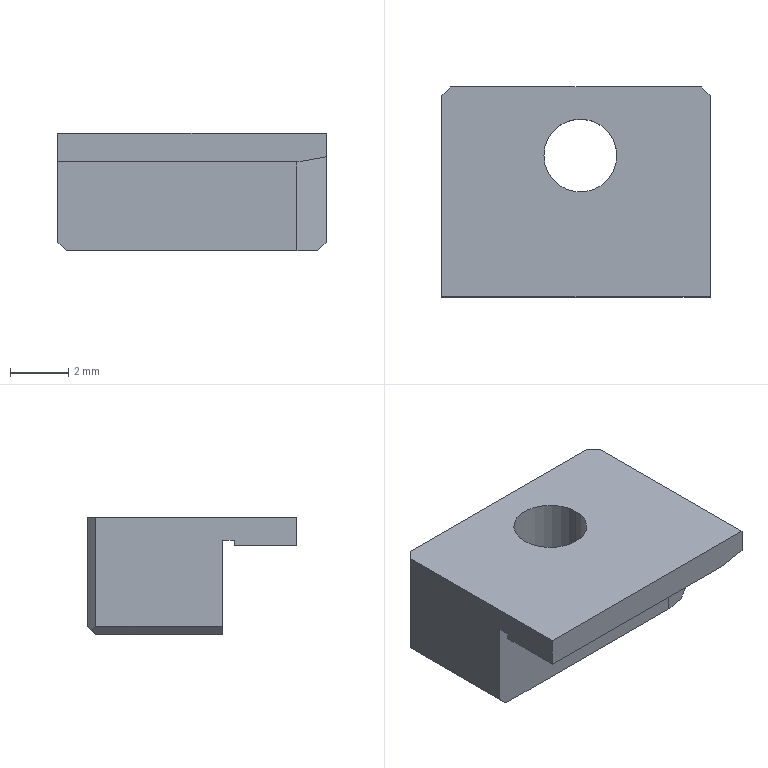Part | NX | 1 solid | 22 faces | box 9.2 x 7.2 x 4.04 mm | volume 173.358 mm3 | plane 18 | cylinder 2 | cone 2 | commonest cylinder face diameters 2.5 x2
STEP:
#1=CARTESIAN_POINT('',(-39.91,-38.279,0.4031));
#2=VERTEX_POINT('',#1);
#3=CARTESIAN_POINT('',(-39.91,-38.279,3.453));
#4=VERTEX_POINT('',#3);
#5=CARTESIAN_POINT('',(-39.91,-38.279,1.928));
#6=DIRECTION('',(0.,0.,1.));
#7=VECTOR('',#6,1000.);
#8=LINE('',#5,#7);
#9=EDGE_CURVE('',#2,#4,#8,.T.);
#10=ORIENTED_EDGE('',*,*,#9,.T.);
#11=CARTESIAN_POINT('',(-38.91,-38.279,3.629));
#12=VERTEX_POINT('',#11);
#13=CARTESIAN_POINT('',(-41.256,-38.279,3.216));
#14=DIRECTION('',(-0.9848,0.,-0.1736));
#15=VECTOR('',#14,1000.);
#16=LINE('',#13,#15);
#17=EDGE_CURVE('',#12,#4,#16,.T.);
#18=ORIENTED_EDGE('',*,*,#17,.F.);
#19=CARTESIAN_POINT('',(-38.91,-38.279,3.653));
#20=VERTEX_POINT('',#19);
#21=CARTESIAN_POINT('',(-38.91,-38.279,3.403));
#22=DIRECTION('',(0.,0.,1.));
#23=VECTOR('',#22,1000.);
#24=LINE('',#21,#23);
#25=EDGE_CURVE('',#12,#20,#24,.T.);
#26=ORIENTED_EDGE('',*,*,#25,.T.);
#27=CARTESIAN_POINT('',(-48.11,-38.279,3.653));
#28=VERTEX_POINT('',#27);
#29=CARTESIAN_POINT('',(-37.99,-38.279,3.653));
#30=DIRECTION('',(-1.,0.,0.));
#31=VECTOR('',#30,1000.);
#32=LINE('',#29,#31);
#33=EDGE_CURVE('',#20,#28,#32,.T.);
#34=ORIENTED_EDGE('',*,*,#33,.T.);
#35=CARTESIAN_POINT('',(-48.11,-38.279,0.7031));
#36=VERTEX_POINT('',#35);
#37=CARTESIAN_POINT('',(-48.11,-38.279,3.403));
#38=DIRECTION('',(0.,0.,1.));
#39=VECTOR('',#38,1000.);
#40=LINE('',#37,#39);
#41=EDGE_CURVE('',#36,#28,#40,.T.);
#42=ORIENTED_EDGE('',*,*,#41,.F.);
#43=CARTESIAN_POINT('',(-47.81,-38.279,0.4031));
#44=VERTEX_POINT('',#43);
#45=CARTESIAN_POINT('',(-50.81,-38.279,3.403));
#46=DIRECTION('',(-0.7071,0.,0.7071));
#47=VECTOR('',#46,1000.);
#48=LINE('',#45,#47);
#49=EDGE_CURVE('',#44,#36,#48,.T.);
#50=ORIENTED_EDGE('',*,*,#49,.F.);
#51=CARTESIAN_POINT('',(-41.256,-38.279,0.4031));
#52=DIRECTION('',(-1.,0.,0.));
#53=VECTOR('',#52,1000.);
#54=LINE('',#51,#53);
#55=EDGE_CURVE('',#2,#44,#54,.T.);
#56=ORIENTED_EDGE('',*,*,#55,.F.);
#57=EDGE_LOOP('',(#10,#18,#26,#34,#42,#50,#56));
#58=FACE_BOUND('',#57,.T.);
#59=CARTESIAN_POINT('',(-48.11,-38.279,3.403));
#60=DIRECTION('',(0.,-1.,0.));
#61=DIRECTION('',(-1.,0.,0.));
#62=AXIS2_PLACEMENT_3D('',#59,#60,#61);
#63=PLANE('',#62);
#64=ADVANCED_FACE('',(#58),#63,.T.);
#65=CARTESIAN_POINT('',(-48.11,-33.929,4.443));
#66=VERTEX_POINT('',#65);
#67=CARTESIAN_POINT('',(-48.11,-40.829,4.443));
#68=VERTEX_POINT('',#67);
#69=CARTESIAN_POINT('',(-48.11,-36.022,4.443));
#70=DIRECTION('',(0.,-1.,0.));
#71=VECTOR('',#70,1000.);
#72=LINE('',#69,#71);
#73=EDGE_CURVE('',#66,#68,#72,.T.);
#74=ORIENTED_EDGE('',*,*,#73,.F.);
#75=CARTESIAN_POINT('',(-48.11,-33.929,0.7031));
#76=VERTEX_POINT('',#75);
#77=CARTESIAN_POINT('',(-48.11,-33.929,3.403));
#78=DIRECTION('',(0.,0.,-1.));
#79=VECTOR('',#78,1000.);
#80=LINE('',#77,#79);
#81=EDGE_CURVE('',#66,#76,#80,.T.);
#82=ORIENTED_EDGE('',*,*,#81,.T.);
#83=CARTESIAN_POINT('',(-48.11,-36.022,0.7031));
#84=DIRECTION('',(0.,1.,0.));
#85=VECTOR('',#84,1000.);
#86=LINE('',#83,#85);
#87=EDGE_CURVE('',#36,#76,#86,.T.);
#88=ORIENTED_EDGE('',*,*,#87,.F.);
#89=ORIENTED_EDGE('',*,*,#41,.T.);
#90=CARTESIAN_POINT('',(-48.11,-38.679,3.653));
#91=VERTEX_POINT('',#90);
#92=CARTESIAN_POINT('',(-48.11,-36.022,3.653));
#93=DIRECTION('',(0.,1.,0.));
#94=VECTOR('',#93,1000.);
#95=LINE('',#92,#94);
#96=EDGE_CURVE('',#91,#28,#95,.T.);
#97=ORIENTED_EDGE('',*,*,#96,.F.);
#98=CARTESIAN_POINT('',(-48.11,-38.679,3.453));
#99=VERTEX_POINT('',#98);
#100=CARTESIAN_POINT('',(-48.11,-38.679,3.403));
#101=DIRECTION('',(0.,0.,1.));
#102=VECTOR('',#101,1000.);
#103=LINE('',#100,#102);
#104=EDGE_CURVE('',#99,#91,#103,.T.);
#105=ORIENTED_EDGE('',*,*,#104,.F.);
#106=CARTESIAN_POINT('',(-48.11,-40.829,3.453));
#107=VERTEX_POINT('',#106);
#108=CARTESIAN_POINT('',(-48.11,-36.022,3.453));
#109=DIRECTION('',(0.,-1.,0.));
#110=VECTOR('',#109,1000.);
#111=LINE('',#108,#110);
#112=EDGE_CURVE('',#99,#107,#111,.T.);
#113=ORIENTED_EDGE('',*,*,#112,.T.);
#114=CARTESIAN_POINT('',(-48.11,-40.829,3.403));
#115=DIRECTION('',(0.,0.,1.));
#116=VECTOR('',#115,1000.);
#117=LINE('',#114,#116);
#118=EDGE_CURVE('',#107,#68,#117,.T.);
#119=ORIENTED_EDGE('',*,*,#118,.T.);
#120=EDGE_LOOP('',(#74,#82,#88,#89,#97,#105,#113,#119));
#121=FACE_BOUND('',#120,.T.);
#122=CARTESIAN_POINT('',(-48.11,-31.629,3.403));
#123=DIRECTION('',(-1.,0.,0.));
#124=DIRECTION('',(0.,1.,0.));
#125=AXIS2_PLACEMENT_3D('',#122,#123,#124);
#126=PLANE('',#125);
#127=ADVANCED_FACE('',(#121),#126,.T.);
#128=CARTESIAN_POINT('',(-39.21,-33.629,4.443));
#129=VERTEX_POINT('',#128);
#130=CARTESIAN_POINT('',(-39.21,-33.629,0.7031));
#131=VERTEX_POINT('',#130);
#132=CARTESIAN_POINT('',(-39.21,-33.629,3.403));
#133=DIRECTION('',(0.,0.,-1.));
#134=VECTOR('',#133,1000.);
#135=LINE('',#132,#134);
#136=EDGE_CURVE('',#129,#131,#135,.T.);
#137=ORIENTED_EDGE('',*,*,#136,.T.);
#138=CARTESIAN_POINT('',(-47.81,-33.629,0.7031));
#139=VERTEX_POINT('',#138);
#140=CARTESIAN_POINT('',(-41.256,-33.629,0.7031));
#141=DIRECTION('',(-1.,0.,0.));
#142=VECTOR('',#141,1000.);
#143=LINE('',#140,#142);
#144=EDGE_CURVE('',#131,#139,#143,.T.);
#145=ORIENTED_EDGE('',*,*,#144,.T.);
#146=CARTESIAN_POINT('',(-47.81,-33.629,4.443));
#147=VERTEX_POINT('',#146);
#148=CARTESIAN_POINT('',(-47.81,-33.629,3.403));
#149=DIRECTION('',(0.,0.,-1.));
#150=VECTOR('',#149,1000.);
#151=LINE('',#148,#150);
#152=EDGE_CURVE('',#147,#139,#151,.T.);
#153=ORIENTED_EDGE('',*,*,#152,.F.);
#154=CARTESIAN_POINT('',(-41.256,-33.629,4.443));
#155=DIRECTION('',(-1.,0.,0.));
#156=VECTOR('',#155,1000.);
#157=LINE('',#154,#156);
#158=EDGE_CURVE('',#129,#147,#157,.T.);
#159=ORIENTED_EDGE('',*,*,#158,.F.);
#160=EDGE_LOOP('',(#137,#145,#153,#159));
#161=FACE_BOUND('',#160,.T.);
#162=CARTESIAN_POINT('',(-38.61,-33.629,3.403));
#163=DIRECTION('',(0.,1.,0.));
#164=DIRECTION('',(1.,0.,0.));
#165=AXIS2_PLACEMENT_3D('',#162,#163,#164);
#166=PLANE('',#165);
#167=ADVANCED_FACE('',(#161),#166,.T.);
#168=CARTESIAN_POINT('',(-38.91,-38.679,3.629));
#169=VERTEX_POINT('',#168);
#170=CARTESIAN_POINT('',(-38.91,-40.829,3.629));
#171=VERTEX_POINT('',#170);
#172=CARTESIAN_POINT('',(-38.91,-39.554,3.629));
#173=DIRECTION('',(0.,-1.,0.));
#174=VECTOR('',#173,1000.);
#175=LINE('',#172,#174);
#176=EDGE_CURVE('',#169,#171,#175,.T.);
#177=ORIENTED_EDGE('',*,*,#176,.F.);
#178=CARTESIAN_POINT('',(-38.91,-38.679,3.653));
#179=VERTEX_POINT('',#178);
#180=CARTESIAN_POINT('',(-38.91,-38.679,3.403));
#181=DIRECTION('',(0.,0.,-1.));
#182=VECTOR('',#181,1000.);
#183=LINE('',#180,#182);
#184=EDGE_CURVE('',#179,#169,#183,.T.);
#185=ORIENTED_EDGE('',*,*,#184,.F.);
#186=CARTESIAN_POINT('',(-38.91,-36.022,3.653));
#187=DIRECTION('',(0.,-1.,0.));
#188=VECTOR('',#187,1000.);
#189=LINE('',#186,#188);
#190=EDGE_CURVE('',#20,#179,#189,.T.);
#191=ORIENTED_EDGE('',*,*,#190,.F.);
#192=ORIENTED_EDGE('',*,*,#25,.F.);
#193=CARTESIAN_POINT('',(-38.91,-38.103,3.629));
#194=VERTEX_POINT('',#193);
#195=CARTESIAN_POINT('',(-38.91,-39.554,3.629));
#196=DIRECTION('',(0.,-1.,0.));
#197=VECTOR('',#196,1000.);
#198=LINE('',#195,#197);
#199=EDGE_CURVE('',#194,#12,#198,.T.);
#200=ORIENTED_EDGE('',*,*,#199,.F.);
#201=CARTESIAN_POINT('',(-38.91,-38.103,0.7031));
#202=VERTEX_POINT('',#201);
#203=CARTESIAN_POINT('',(-38.91,-38.103,1.928));
#204=DIRECTION('',(0.,0.,1.));
#205=VECTOR('',#204,1000.);
#206=LINE('',#203,#205);
#207=EDGE_CURVE('',#202,#194,#206,.T.);
#208=ORIENTED_EDGE('',*,*,#207,.F.);
#209=CARTESIAN_POINT('',(-38.91,-33.929,0.7031));
#210=VERTEX_POINT('',#209);
#211=CARTESIAN_POINT('',(-38.91,-36.104,0.7031));
#212=DIRECTION('',(0.,-1.,0.));
#213=VECTOR('',#212,1000.);
#214=LINE('',#211,#213);
#215=EDGE_CURVE('',#210,#202,#214,.T.);
#216=ORIENTED_EDGE('',*,*,#215,.F.);
#217=CARTESIAN_POINT('',(-38.91,-33.929,4.443));
#218=VERTEX_POINT('',#217);
#219=CARTESIAN_POINT('',(-38.91,-33.929,3.403));
#220=DIRECTION('',(0.,0.,-1.));
#221=VECTOR('',#220,1000.);
#222=LINE('',#219,#221);
#223=EDGE_CURVE('',#218,#210,#222,.T.);
#224=ORIENTED_EDGE('',*,*,#223,.F.);
#225=CARTESIAN_POINT('',(-38.91,-40.829,4.443));
#226=VERTEX_POINT('',#225);
#227=CARTESIAN_POINT('',(-38.91,-36.022,4.443));
#228=DIRECTION('',(0.,1.,0.));
#229=VECTOR('',#228,1000.);
#230=LINE('',#227,#229);
#231=EDGE_CURVE('',#226,#218,#230,.T.);
#232=ORIENTED_EDGE('',*,*,#231,.F.);
#233=CARTESIAN_POINT('',(-38.91,-40.829,3.403));
#234=DIRECTION('',(0.,0.,1.));
#235=VECTOR('',#234,1000.);
#236=LINE('',#233,#235);
#237=EDGE_CURVE('',#171,#226,#236,.T.);
#238=ORIENTED_EDGE('',*,*,#237,.F.);
#239=EDGE_LOOP('',(#177,#185,#191,#192,#200,#208,#216,#224,#232,#238));
#240=FACE_BOUND('',#239,.T.);
#241=CARTESIAN_POINT('',(-38.91,-38.329,3.403));
#242=DIRECTION('',(1.,0.,0.));
#243=DIRECTION('',(0.,0.,1.));
#244=AXIS2_PLACEMENT_3D('',#241,#242,#243);
#245=PLANE('',#244);
#246=ADVANCED_FACE('',(#240),#245,.T.);
#247=CARTESIAN_POINT('',(-41.256,-27.074,4.443));
#248=DIRECTION('',(-0.7071,-0.7071,0.));
#249=VECTOR('',#248,1000.);
#250=LINE('',#247,#249);
#251=EDGE_CURVE('',#147,#66,#250,.T.);
#252=ORIENTED_EDGE('',*,*,#251,.F.);
#253=ORIENTED_EDGE('',*,*,#152,.T.);
#254=CARTESIAN_POINT('',(-47.96,-33.779,0.5531));
#255=VERTEX_POINT('',#254);
#256=CARTESIAN_POINT('',(-41.256,-27.074,7.258));
#257=DIRECTION('',(-0.5774,-0.5774,-0.5774));
#258=VECTOR('',#257,1000.);
#259=LINE('',#256,#258);
#260=EDGE_CURVE('',#139,#255,#259,.T.);
#261=ORIENTED_EDGE('',*,*,#260,.T.);
#262=CARTESIAN_POINT('',(-50.81,-36.629,3.403));
#263=DIRECTION('',(0.5774,0.5774,-0.5774));
#264=VECTOR('',#263,1000.);
#265=LINE('',#262,#264);
#266=EDGE_CURVE('',#76,#255,#265,.T.);
#267=ORIENTED_EDGE('',*,*,#266,.F.);
#268=ORIENTED_EDGE('',*,*,#81,.F.);
#269=EDGE_LOOP('',(#252,#253,#261,#267,#268));
#270=FACE_BOUND('',#269,.T.);
#271=CARTESIAN_POINT('',(-47.96,-33.779,2.553));
#272=DIRECTION('',(-0.7071,0.7071,0.));
#273=DIRECTION('',(0.,0.,1.));
#274=AXIS2_PLACEMENT_3D('',#271,#272,#273);
#275=PLANE('',#274);
#276=ADVANCED_FACE('',(#270),#275,.T.);
#277=ORIENTED_EDGE('',*,*,#17,.T.);
#278=CARTESIAN_POINT('',(-41.256,-38.516,3.216));
#279=DIRECTION('',(0.9703,0.1711,0.1711));
#280=VECTOR('',#279,1000.);
#281=LINE('',#278,#280);
#282=EDGE_CURVE('',#4,#194,#281,.T.);
#283=ORIENTED_EDGE('',*,*,#282,.T.);
#284=ORIENTED_EDGE('',*,*,#199,.T.);
#285=EDGE_LOOP('',(#277,#283,#284));
#286=FACE_BOUND('',#285,.T.);
#287=CARTESIAN_POINT('',(-39.41,-39.554,3.541));
#288=DIRECTION('',(-0.1736,0.,0.9848));
#289=DIRECTION('',(0.,1.,0.));
#290=AXIS2_PLACEMENT_3D('',#287,#288,#289);
#291=PLANE('',#290);
#292=ADVANCED_FACE('',(#286),#291,.F.);
#293=CARTESIAN_POINT('',(-41.256,-40.829,4.443));
#294=DIRECTION('',(1.,0.,0.));
#295=VECTOR('',#294,1000.);
#296=LINE('',#293,#295);
#297=EDGE_CURVE('',#68,#226,#296,.T.);
#298=ORIENTED_EDGE('',*,*,#297,.F.);
#299=ORIENTED_EDGE('',*,*,#118,.F.);
#300=CARTESIAN_POINT('',(-39.91,-40.829,3.453));
#301=VERTEX_POINT('',#300);
#302=CARTESIAN_POINT('',(-41.256,-40.829,3.453));
#303=DIRECTION('',(-1.,0.,0.));
#304=VECTOR('',#303,1000.);
#305=LINE('',#302,#304);
#306=EDGE_CURVE('',#301,#107,#305,.T.);
#307=ORIENTED_EDGE('',*,*,#306,.F.);
#308=CARTESIAN_POINT('',(-41.256,-40.829,3.216));
#309=DIRECTION('',(0.9848,0.,0.1736));
#310=VECTOR('',#309,1000.);
#311=LINE('',#308,#310);
#312=EDGE_CURVE('',#301,#171,#311,.T.);
#313=ORIENTED_EDGE('',*,*,#312,.T.);
#314=ORIENTED_EDGE('',*,*,#237,.T.);
#315=EDGE_LOOP('',(#298,#299,#307,#313,#314));
#316=FACE_BOUND('',#315,.T.);
#317=CARTESIAN_POINT('',(-43.439,-40.829,4.035));
#318=DIRECTION('',(0.,-1.,0.));
#319=DIRECTION('',(-1.,0.,0.));
#320=AXIS2_PLACEMENT_3D('',#317,#318,#319);
#321=PLANE('',#320);
#322=ADVANCED_FACE('',(#316),#321,.T.);
#323=ORIENTED_EDGE('',*,*,#176,.T.);
#324=ORIENTED_EDGE('',*,*,#312,.F.);
#325=CARTESIAN_POINT('',(-39.91,-38.679,3.453));
#326=VERTEX_POINT('',#325);
#327=CARTESIAN_POINT('',(-39.91,-39.554,3.453));
#328=DIRECTION('',(0.,-1.,0.));
#329=VECTOR('',#328,1000.);
#330=LINE('',#327,#329);
#331=EDGE_CURVE('',#326,#301,#330,.T.);
#332=ORIENTED_EDGE('',*,*,#331,.F.);
#333=CARTESIAN_POINT('',(-41.256,-38.679,3.216));
#334=DIRECTION('',(0.9848,0.,0.1736));
#335=VECTOR('',#334,1000.);
#336=LINE('',#333,#335);
#337=EDGE_CURVE('',#326,#169,#336,.T.);
#338=ORIENTED_EDGE('',*,*,#337,.T.);
#339=EDGE_LOOP('',(#323,#324,#332,#338));
#340=FACE_BOUND('',#339,.T.);
#341=CARTESIAN_POINT('',(-39.41,-39.554,3.541));
#342=DIRECTION('',(-0.1736,0.,0.9848));
#343=DIRECTION('',(0.,1.,0.));
#344=AXIS2_PLACEMENT_3D('',#341,#342,#343);
#345=PLANE('',#344);
#346=ADVANCED_FACE('',(#340),#345,.F.);
#347=ORIENTED_EDGE('',*,*,#9,.F.);
#348=CARTESIAN_POINT('',(-39.21,-38.156,0.4031));
#349=VERTEX_POINT('',#348);
#350=CARTESIAN_POINT('',(-41.256,-38.516,0.4031));
#351=DIRECTION('',(0.9848,0.1736,0.));
#352=VECTOR('',#351,1000.);
#353=LINE('',#350,#352);
#354=EDGE_CURVE('',#2,#349,#353,.T.);
#355=ORIENTED_EDGE('',*,*,#354,.T.);
#356=CARTESIAN_POINT('',(-36.21,-37.627,3.403));
#357=DIRECTION('',(0.7017,0.1237,0.7017));
#358=VECTOR('',#357,1000.);
#359=LINE('',#356,#358);
#360=EDGE_CURVE('',#349,#202,#359,.T.);
#361=ORIENTED_EDGE('',*,*,#360,.T.);
#362=ORIENTED_EDGE('',*,*,#207,.T.);
#363=ORIENTED_EDGE('',*,*,#282,.F.);
#364=EDGE_LOOP('',(#347,#355,#361,#362,#363));
#365=FACE_BOUND('',#364,.T.);
#366=CARTESIAN_POINT('',(-39.41,-38.191,1.928));
#367=DIRECTION('',(0.1736,-0.9848,0.));
#368=DIRECTION('',(0.,0.,-1.));
#369=AXIS2_PLACEMENT_3D('',#366,#367,#368);
#370=PLANE('',#369);
#371=ADVANCED_FACE('',(#365),#370,.T.);
#372=ORIENTED_EDGE('',*,*,#136,.F.);
#373=CARTESIAN_POINT('',(-36.817,-36.022,4.443));
#374=DIRECTION('',(-0.7071,0.7071,0.));
#375=VECTOR('',#374,1000.);
#376=LINE('',#373,#375);
#377=EDGE_CURVE('',#218,#129,#376,.T.);
#378=ORIENTED_EDGE('',*,*,#377,.F.);
#379=ORIENTED_EDGE('',*,*,#223,.T.);
#380=CARTESIAN_POINT('',(-39.06,-33.779,0.5531));
#381=VERTEX_POINT('',#380);
#382=CARTESIAN_POINT('',(-36.817,-36.022,2.796));
#383=DIRECTION('',(-0.5774,0.5774,-0.5774));
#384=VECTOR('',#383,1000.);
#385=LINE('',#382,#384);
#386=EDGE_CURVE('',#210,#381,#385,.T.);
#387=ORIENTED_EDGE('',*,*,#386,.T.);
#388=CARTESIAN_POINT('',(-36.817,-36.022,-1.69));
#389=DIRECTION('',(0.5774,-0.5774,-0.5774));
#390=VECTOR('',#389,1000.);
#391=LINE('',#388,#390);
#392=EDGE_CURVE('',#131,#381,#391,.T.);
#393=ORIENTED_EDGE('',*,*,#392,.F.);
#394=EDGE_LOOP('',(#372,#378,#379,#387,#393));
#395=FACE_BOUND('',#394,.T.);
#396=CARTESIAN_POINT('',(-39.06,-33.779,2.553));
#397=DIRECTION('',(0.7071,0.7071,0.));
#398=DIRECTION('',(0.,0.,-1.));
#399=AXIS2_PLACEMENT_3D('',#396,#397,#398);
#400=PLANE('',#399);
#401=ADVANCED_FACE('',(#395),#400,.T.);
#402=CARTESIAN_POINT('',(-41.256,-38.679,3.453));
#403=DIRECTION('',(-1.,0.,0.));
#404=VECTOR('',#403,1000.);
#405=LINE('',#402,#404);
#406=EDGE_CURVE('',#326,#99,#405,.T.);
#407=ORIENTED_EDGE('',*,*,#406,.F.);
#408=ORIENTED_EDGE('',*,*,#331,.T.);
#409=ORIENTED_EDGE('',*,*,#306,.T.);
#410=ORIENTED_EDGE('',*,*,#112,.F.);
#411=EDGE_LOOP('',(#407,#408,#409,#410));
#412=FACE_BOUND('',#411,.T.);
#413=CARTESIAN_POINT('',(-38.61,-38.329,3.453));
#414=DIRECTION('',(0.,0.,-1.));
#415=DIRECTION('',(0.,-1.,0.));
#416=AXIS2_PLACEMENT_3D('',#413,#414,#415);
#417=PLANE('',#416);
#418=ADVANCED_FACE('',(#412),#417,.T.);
#419=ORIENTED_EDGE('',*,*,#184,.T.);
#420=ORIENTED_EDGE('',*,*,#337,.F.);
#421=ORIENTED_EDGE('',*,*,#406,.T.);
#422=ORIENTED_EDGE('',*,*,#104,.T.);
#423=CARTESIAN_POINT('',(-37.99,-38.679,3.653));
#424=DIRECTION('',(-1.,0.,0.));
#425=VECTOR('',#424,1000.);
#426=LINE('',#423,#425);
#427=EDGE_CURVE('',#179,#91,#426,.T.);
#428=ORIENTED_EDGE('',*,*,#427,.F.);
#429=EDGE_LOOP('',(#419,#420,#421,#422,#428));
#430=FACE_BOUND('',#429,.T.);
#431=CARTESIAN_POINT('',(-37.99,-38.679,3.653));
#432=DIRECTION('',(0.,-1.,0.));
#433=DIRECTION('',(0.,0.,-1.));
#434=AXIS2_PLACEMENT_3D('',#431,#432,#433);
#435=PLANE('',#434);
#436=ADVANCED_FACE('',(#430),#435,.F.);
#437=ORIENTED_EDGE('',*,*,#190,.T.);
#438=ORIENTED_EDGE('',*,*,#427,.T.);
#439=ORIENTED_EDGE('',*,*,#96,.T.);
#440=ORIENTED_EDGE('',*,*,#33,.F.);
#441=EDGE_LOOP('',(#437,#438,#439,#440));
#442=FACE_BOUND('',#441,.T.);
#443=CARTESIAN_POINT('',(-37.99,-38.279,3.653));
#444=DIRECTION('',(0.,0.,1.));
#445=DIRECTION('',(1.,0.,0.));
#446=AXIS2_PLACEMENT_3D('',#443,#444,#445);
#447=PLANE('',#446);
#448=ADVANCED_FACE('',(#442),#447,.F.);
#449=CARTESIAN_POINT('',(-39.21,-33.929,0.4031));
#450=VERTEX_POINT('',#449);
#451=CARTESIAN_POINT('',(-39.21,-36.104,0.4031));
#452=DIRECTION('',(0.,-1.,0.));
#453=VECTOR('',#452,1000.);
#454=LINE('',#451,#453);
#455=EDGE_CURVE('',#450,#349,#454,.T.);
#456=ORIENTED_EDGE('',*,*,#455,.T.);
#457=ORIENTED_EDGE('',*,*,#354,.F.);
#458=ORIENTED_EDGE('',*,*,#55,.T.);
#459=CARTESIAN_POINT('',(-47.81,-33.929,0.4031));
#460=VERTEX_POINT('',#459);
#461=CARTESIAN_POINT('',(-47.81,-36.022,0.4031));
#462=DIRECTION('',(0.,1.,0.));
#463=VECTOR('',#462,1000.);
#464=LINE('',#461,#463);
#465=EDGE_CURVE('',#44,#460,#464,.T.);
#466=ORIENTED_EDGE('',*,*,#465,.T.);
#467=CARTESIAN_POINT('',(-41.256,-33.929,0.4031));
#468=DIRECTION('',(-1.,0.,0.));
#469=VECTOR('',#468,1000.);
#470=LINE('',#467,#469);
#471=EDGE_CURVE('',#450,#460,#470,.T.);
#472=ORIENTED_EDGE('',*,*,#471,.F.);
#473=EDGE_LOOP('',(#456,#457,#458,#466,#472));
#474=FACE_BOUND('',#473,.T.);
#475=CARTESIAN_POINT('',(-41.66,-35.979,0.4031));
#476=VERTEX_POINT('',#475);
#477=CARTESIAN_POINT('',(-45.06,-35.979,0.4031));
#478=VERTEX_POINT('',#477);
#479=CARTESIAN_POINT('',(-43.36,-35.979,0.4031));
#480=DIRECTION('',(0.,0.,-1.));
#481=DIRECTION('',(-1.,0.,0.));
#482=AXIS2_PLACEMENT_3D('',#479,#480,#481);
#483=CIRCLE('',#482,1.7);
#484=EDGE_CURVE('',#476,#478,#483,.T.);
#485=ORIENTED_EDGE('',*,*,#484,.F.);
#486=CARTESIAN_POINT('',(-43.36,-35.979,0.4031));
#487=DIRECTION('',(0.,0.,-1.));
#488=DIRECTION('',(-1.,0.,0.));
#489=AXIS2_PLACEMENT_3D('',#486,#487,#488);
#490=CIRCLE('',#489,1.7);
#491=EDGE_CURVE('',#478,#476,#490,.T.);
#492=ORIENTED_EDGE('',*,*,#491,.F.);
#493=EDGE_LOOP('',(#485,#492));
#494=FACE_BOUND('',#493,.T.);
#495=CARTESIAN_POINT('',(-41.256,-36.022,0.4031));
#496=DIRECTION('',(0.,0.,-1.));
#497=DIRECTION('',(0.,-1.,0.));
#498=AXIS2_PLACEMENT_3D('',#495,#496,#497);
#499=PLANE('',#498);
#500=ADVANCED_FACE('',(#474,#494),#499,.T.);
#501=CARTESIAN_POINT('',(-42.11,-35.979,0.6629));
#502=VERTEX_POINT('',#501);
#503=CARTESIAN_POINT('',(-44.61,-35.979,0.6629));
#504=VERTEX_POINT('',#503);
#505=CARTESIAN_POINT('',(-43.36,-35.979,0.6629));
#506=DIRECTION('',(0.,0.,-1.));
#507=DIRECTION('',(-1.,0.,0.));
#508=AXIS2_PLACEMENT_3D('',#505,#506,#507);
#509=CIRCLE('',#508,1.25);
#510=EDGE_CURVE('',#502,#504,#509,.T.);
#511=ORIENTED_EDGE('',*,*,#510,.T.);
#512=CARTESIAN_POINT('',(-44.61,-35.979,4.443));
#513=VERTEX_POINT('',#512);
#514=CARTESIAN_POINT('',(-44.61,-35.979,0.4031));
#515=DIRECTION('',(0.,0.,-1.));
#516=VECTOR('',#515,1000.);
#517=LINE('',#514,#516);
#518=EDGE_CURVE('',#504,#513,#517,.F.);
#519=ORIENTED_EDGE('',*,*,#518,.T.);
#520=CARTESIAN_POINT('',(-42.11,-35.979,4.443));
#521=VERTEX_POINT('',#520);
#522=CARTESIAN_POINT('',(-43.36,-35.979,4.443));
#523=DIRECTION('',(0.,0.,-1.));
#524=DIRECTION('',(-1.,0.,0.));
#525=AXIS2_PLACEMENT_3D('',#522,#523,#524);
#526=CIRCLE('',#525,1.25);
#527=EDGE_CURVE('',#521,#513,#526,.T.);
#528=ORIENTED_EDGE('',*,*,#527,.F.);
#529=CARTESIAN_POINT('',(-42.11,-35.979,0.4031));
#530=DIRECTION('',(0.,0.,-1.));
#531=VECTOR('',#530,1000.);
#532=LINE('',#529,#531);
#533=EDGE_CURVE('',#502,#521,#532,.F.);
#534=ORIENTED_EDGE('',*,*,#533,.F.);
#535=EDGE_LOOP('',(#511,#519,#528,#534));
#536=FACE_BOUND('',#535,.T.);
#537=CARTESIAN_POINT('',(-43.36,-35.979,0.4031));
#538=DIRECTION('',(0.,0.,-1.));
#539=DIRECTION('',(-1.,0.,0.));
#540=AXIS2_PLACEMENT_3D('',#537,#538,#539);
#541=CYLINDRICAL_SURFACE('',#540,1.25);
#542=ADVANCED_FACE('',(#536),#541,.F.);
#543=ORIENTED_EDGE('',*,*,#144,.F.);
#544=ORIENTED_EDGE('',*,*,#392,.T.);
#545=CARTESIAN_POINT('',(-36.21,-30.929,3.403));
#546=DIRECTION('',(-0.5774,-0.5774,-0.5774));
#547=VECTOR('',#546,1000.);
#548=LINE('',#545,#547);
#549=EDGE_CURVE('',#381,#450,#548,.T.);
#550=ORIENTED_EDGE('',*,*,#549,.T.);
#551=ORIENTED_EDGE('',*,*,#471,.T.);
#552=CARTESIAN_POINT('',(-45.717,-36.022,-1.69));
#553=DIRECTION('',(-0.5774,0.5774,0.5774));
#554=VECTOR('',#553,1000.);
#555=LINE('',#552,#554);
#556=EDGE_CURVE('',#460,#255,#555,.T.);
#557=ORIENTED_EDGE('',*,*,#556,.T.);
#558=ORIENTED_EDGE('',*,*,#260,.F.);
#559=EDGE_LOOP('',(#543,#544,#550,#551,#557,#558));
#560=FACE_BOUND('',#559,.T.);
#561=CARTESIAN_POINT('',(-43.36,-33.779,0.5531));
#562=DIRECTION('',(0.,-0.7071,0.7071));
#563=DIRECTION('',(-1.,0.,0.));
#564=AXIS2_PLACEMENT_3D('',#561,#562,#563);
#565=PLANE('',#564);
#566=ADVANCED_FACE('',(#560),#565,.F.);
#567=ORIENTED_EDGE('',*,*,#510,.F.);
#568=CARTESIAN_POINT('',(-42.11,-35.979,0.6629));
#569=DIRECTION('',(0.866,0.,-0.5));
#570=VECTOR('',#569,1000.);
#571=LINE('',#568,#570);
#572=EDGE_CURVE('',#476,#502,#571,.F.);
#573=ORIENTED_EDGE('',*,*,#572,.F.);
#574=ORIENTED_EDGE('',*,*,#484,.T.);
#575=CARTESIAN_POINT('',(-44.61,-35.979,0.6629));
#576=DIRECTION('',(-0.866,0.,-0.5));
#577=VECTOR('',#576,1000.);
#578=LINE('',#575,#577);
#579=EDGE_CURVE('',#478,#504,#578,.F.);
#580=ORIENTED_EDGE('',*,*,#579,.T.);
#581=EDGE_LOOP('',(#567,#573,#574,#580));
#582=FACE_BOUND('',#581,.T.);
#583=CARTESIAN_POINT('',(-43.36,-35.979,0.6629));
#584=DIRECTION('',(0.,0.,-1.));
#585=DIRECTION('',(-1.,0.,0.));
#586=AXIS2_PLACEMENT_3D('',#583,#584,#585);
#587=CONICAL_SURFACE('',#586,1.25,1.047);
#588=ADVANCED_FACE('',(#582),#587,.F.);
#589=ORIENTED_EDGE('',*,*,#465,.F.);
#590=ORIENTED_EDGE('',*,*,#49,.T.);
#591=ORIENTED_EDGE('',*,*,#87,.T.);
#592=ORIENTED_EDGE('',*,*,#266,.T.);
#593=ORIENTED_EDGE('',*,*,#556,.F.);
#594=EDGE_LOOP('',(#589,#590,#591,#592,#593));
#595=FACE_BOUND('',#594,.T.);
#596=CARTESIAN_POINT('',(-47.96,-36.129,0.5531));
#597=DIRECTION('',(-0.7071,0.,-0.7071));
#598=DIRECTION('',(-0.7071,0.,0.7071));
#599=AXIS2_PLACEMENT_3D('',#596,#597,#598);
#600=PLANE('',#599);
#601=ADVANCED_FACE('',(#595),#600,.T.);
#602=ORIENTED_EDGE('',*,*,#455,.F.);
#603=ORIENTED_EDGE('',*,*,#549,.F.);
#604=ORIENTED_EDGE('',*,*,#386,.F.);
#605=ORIENTED_EDGE('',*,*,#215,.T.);
#606=ORIENTED_EDGE('',*,*,#360,.F.);
#607=EDGE_LOOP('',(#602,#603,#604,#605,#606));
#608=FACE_BOUND('',#607,.T.);
#609=CARTESIAN_POINT('',(-39.06,-36.104,0.5531));
#610=DIRECTION('',(0.7071,0.,-0.7071));
#611=DIRECTION('',(0.,-1.,0.));
#612=AXIS2_PLACEMENT_3D('',#609,#610,#611);
#613=PLANE('',#612);
#614=ADVANCED_FACE('',(#608),#613,.T.);
#615=ORIENTED_EDGE('',*,*,#518,.F.);
#616=CARTESIAN_POINT('',(-43.36,-35.979,0.6629));
#617=DIRECTION('',(0.,0.,-1.));
#618=DIRECTION('',(-1.,0.,0.));
#619=AXIS2_PLACEMENT_3D('',#616,#617,#618);
#620=CIRCLE('',#619,1.25);
#621=EDGE_CURVE('',#504,#502,#620,.T.);
#622=ORIENTED_EDGE('',*,*,#621,.T.);
#623=ORIENTED_EDGE('',*,*,#533,.T.);
#624=CARTESIAN_POINT('',(-43.36,-35.979,4.443));
#625=DIRECTION('',(0.,0.,-1.));
#626=DIRECTION('',(-1.,0.,0.));
#627=AXIS2_PLACEMENT_3D('',#624,#625,#626);
#628=CIRCLE('',#627,1.25);
#629=EDGE_CURVE('',#513,#521,#628,.T.);
#630=ORIENTED_EDGE('',*,*,#629,.F.);
#631=EDGE_LOOP('',(#615,#622,#623,#630));
#632=FACE_BOUND('',#631,.T.);
#633=CARTESIAN_POINT('',(-43.36,-35.979,0.4031));
#634=DIRECTION('',(0.,0.,-1.));
#635=DIRECTION('',(-1.,0.,0.));
#636=AXIS2_PLACEMENT_3D('',#633,#634,#635);
#637=CYLINDRICAL_SURFACE('',#636,1.25);
#638=ADVANCED_FACE('',(#632),#637,.F.);
#639=ORIENTED_EDGE('',*,*,#579,.F.);
#640=ORIENTED_EDGE('',*,*,#491,.T.);
#641=ORIENTED_EDGE('',*,*,#572,.T.);
#642=ORIENTED_EDGE('',*,*,#621,.F.);
#643=EDGE_LOOP('',(#639,#640,#641,#642));
#644=FACE_BOUND('',#643,.T.);
#645=CARTESIAN_POINT('',(-43.36,-35.979,0.6629));
#646=DIRECTION('',(0.,0.,-1.));
#647=DIRECTION('',(-1.,0.,0.));
#648=AXIS2_PLACEMENT_3D('',#645,#646,#647);
#649=CONICAL_SURFACE('',#648,1.25,1.047);
#650=ADVANCED_FACE('',(#644),#649,.F.);
#651=ORIENTED_EDGE('',*,*,#231,.T.);
#652=ORIENTED_EDGE('',*,*,#377,.T.);
#653=ORIENTED_EDGE('',*,*,#158,.T.);
#654=ORIENTED_EDGE('',*,*,#251,.T.);
#655=ORIENTED_EDGE('',*,*,#73,.T.);
#656=ORIENTED_EDGE('',*,*,#297,.T.);
#657=EDGE_LOOP('',(#651,#652,#653,#654,#655,#656));
#658=FACE_BOUND('',#657,.T.);
#659=ORIENTED_EDGE('',*,*,#527,.T.);
#660=ORIENTED_EDGE('',*,*,#629,.T.);
#661=EDGE_LOOP('',(#659,#660));
#662=FACE_BOUND('',#661,.T.);
#663=CARTESIAN_POINT('',(-41.256,-36.022,4.443));
#664=DIRECTION('',(0.,0.,-1.));
#665=DIRECTION('',(0.,-1.,0.));
#666=AXIS2_PLACEMENT_3D('',#663,#664,#665);
#667=PLANE('',#666);
#668=ADVANCED_FACE('',(#658,#662),#667,.F.);
#669=CLOSED_SHELL('',(#64,#127,#167,#246,#276,#292,#322,#346,#371,#401,#418,#436,#448,#500,#542,#566,#588,#601,#614,#638,#650,#668));
#670=MANIFOLD_SOLID_BREP('',#669);
#671=(LENGTH_UNIT()NAMED_UNIT(*)SI_UNIT(.MILLI.,.METRE.));
#672=UNCERTAINTY_MEASURE_WITH_UNIT(LENGTH_MEASURE(0.00001),#671,'','');
#673=(NAMED_UNIT(*)PLANE_ANGLE_UNIT()SI_UNIT($,.RADIAN.));
#674=(NAMED_UNIT(*)SI_UNIT($,.STERADIAN.)SOLID_ANGLE_UNIT());
#675=(GEOMETRIC_REPRESENTATION_CONTEXT(3)GLOBAL_UNCERTAINTY_ASSIGNED_CONTEXT((#672))GLOBAL_UNIT_ASSIGNED_CONTEXT((#671,#673,#674))REPRESENTATION_CONTEXT('',''));
#676=ADVANCED_BREP_SHAPE_REPRESENTATION('',(#670),#675);